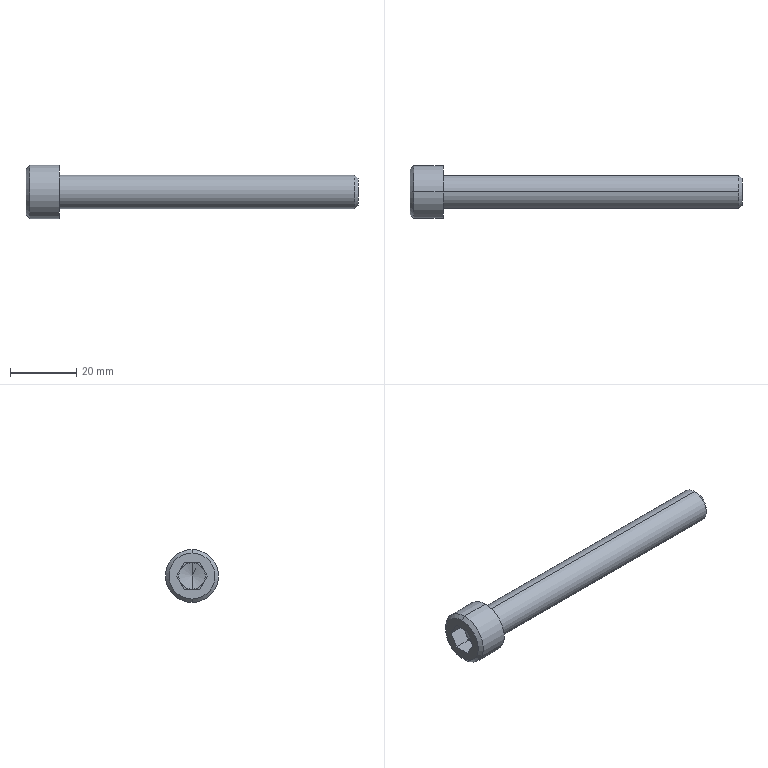Part | STEP file | 0245_033_ASCB10-90 | 1 solid | 25 faces | box 100 x 16 x 16 mm | volume 8744 mm3 | plane 15 | cone 6 | cylinder 4 | commonest cylinder face diameters 10 x2 16 x2